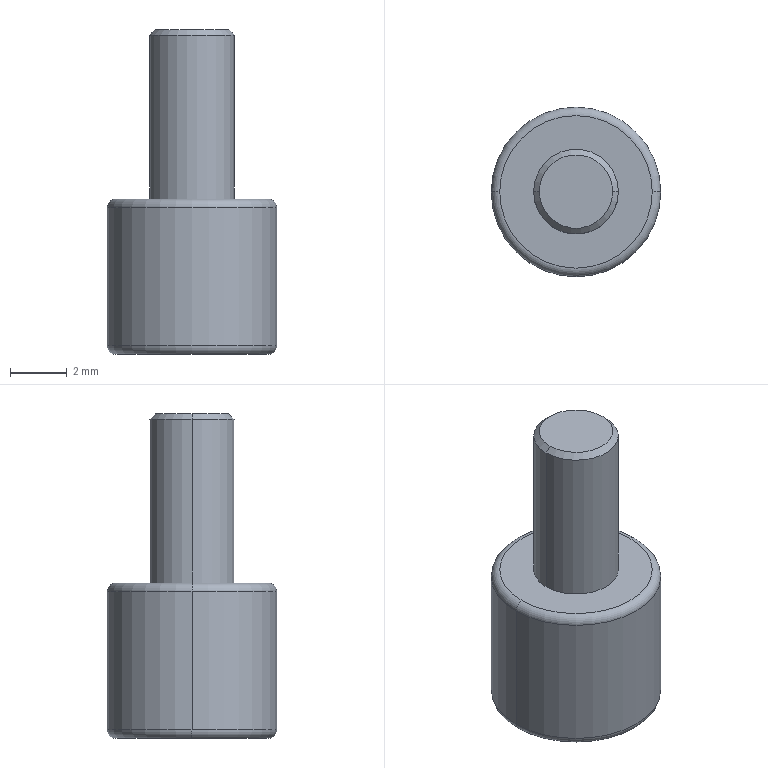Part | STEP file | QA-CFM3-6 | 1 solid | 24 faces | box 6 x 6 x 11.5 mm | volume 192.07 mm3 | plane 10 | cylinder 6 | cone 4 | torus 4 | commonest cylinder face diameters 2 x2 3 x2 6 x2